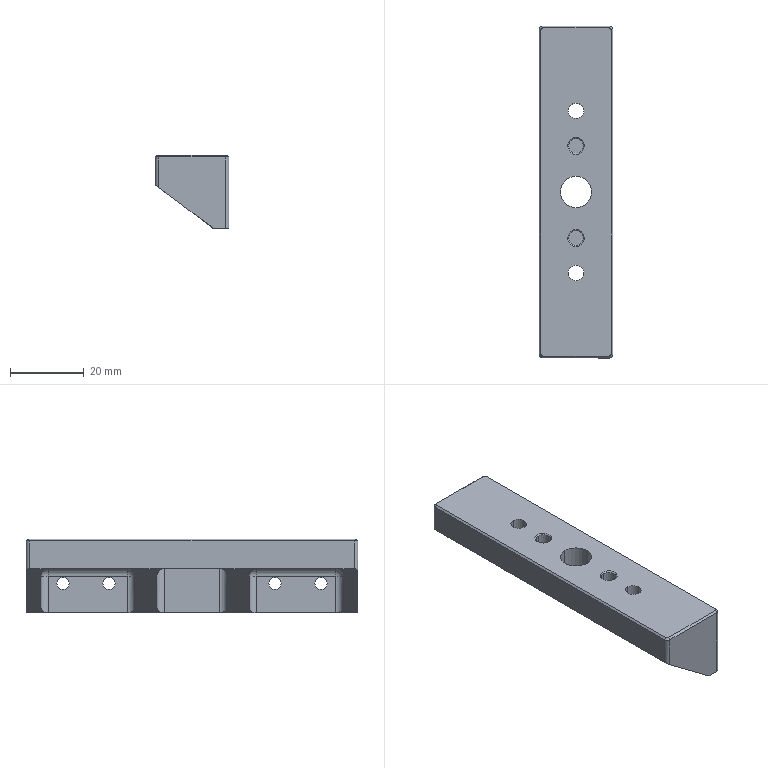NC program | NX | posted with a generic post | part box 20 x 90 x 20 mm
Whole program:
N10 G17 G21 G94 G90
(FLOOR_WALL , TOOL : D80)
N12 T19 M6
N14 G54
N16 G17 G0 G90 X93. Y0. B0. C0. S6500 M3
N18 G43 Z30. H19
N20 Z3.
N22 G94 G1 Z0. F1500.
N24 X90.
N26 X-90.
N28 X-93.
N30 Z3.
N32 G0 Z30.
N34 M5
(DRILLING_COPY_1 , TOOL : D6A45)
N36 T01 M6
N38 G54
N40 G17 G0 G90 X-22. Y0. B0. C0. S5000 M3
N42 G43 Z30. H1
N44 G94 G81 G98 Z-2.3 F350. R3.
N46 X-12.5
N48 X0.
N50 X12.5
N52 X22.
N54 G80
N56 G0 X22. Y0. Z30.
N58 M5
(DRILLING_COPY_COPY , TOOL : 4.2ZT)
N60 T04 M6
N62 G54
N64 G17 G0 G90 X-22. Y0. B0. C0. S2000 M3
N66 G43 Z30. H4
N68 G94 G83 G98 Z-12.262 F180. Q2. R3.
N70 X22.
N72 G80
N74 G0 X22. Y0. Z30.
N76 M5
(ADAPTIVE_MILLING , TOOL : D10)
N78 T15 M6
N80 G54
N82 G17 G0 G90 X0.062 Y-22.709 B0. C0. S9500 M3
N84 G43 Z30. H15
N86 Z-17.
N88 G94 G1 Z-20. F1000.
N90 X0.341 Y-21.928 F3000.
N92 X0.598 Y-21.14
N94 G3 X0.062 Y-20.062 R1.017
N96 X-3.002 Y-19.301 R8.28
N98 X-12.869 Y-19.018 R111.643
N100 G1 X-15.119 Y-19.014
N102 X-18.994 Y-19.011
N104 X-32.619 Y-19.01
N106 X-46.869
N108 X-46.994 Y-19.009
N110 X-47.119 Y-19.007
N112 G2 X-51.4 Y-16.514 R5.714
N114 X-53.465 Y-11.074 R12.318
N116 X-53.953 Y-2.971 R57.395
N118 X-53.956 Y12.528 R542.605
N120 X-51.057 Y16.709 R6.079
N122 X-45.402 Y18.564 R13.739
N124 X-36.541 Y18.967 R76.862
N126 G1 X-35.166 Y18.975
N128 X-33.416 Y18.981
N130 X-30.791 Y18.985
N132 X-25.916 Y18.987
N134 X46.959 Y18.988
N136 X47.084 Y18.987
N138 G2 X51.303 Y16.62 R5.659
N140 X53.46 Y11.087 R12.126
N142 X53.952 Y2.985 R56.695
N144 X53.957 Y-12.514 R598.469
N146 X51.067 Y-16.7 R6.069
N148 X45.414 Y-18.561 R13.651
N150 X36.679 Y-18.965 R74.648
N152 G1 X35.304 Y-18.974
N154 X33.554 Y-18.98
N156 X31.054 Y-18.985
N158 X26.554 Y-18.987
N160 X3.804 Y-18.988
N162 X3.679 Y-18.987
N164 G2 X-1.917 Y-18.439 R78.95
N166 G3 X-14.656 Y-18.033 R144.53
N168 G1 X-16.906 Y-18.027
N170 X-20.156 Y-18.023
N172 X-26.656 Y-18.021
N174 X-43.906 Y-18.02
N176 X-44.031 Y-18.019
N178 X-44.156 Y-18.016
N180 G2 X-50.337 Y-14.316 R7.67
N182 X-52.487 Y-7.845 R15.641
N184 X-52.943 Y1.013 R73.919
N186 X-52.943 Y9.637 R305.783
N188 X-49.084 Y15.462 R7.751
N190 X-42.579 Y17.519 R16.188
N192 X-32.594 Y17.955 R89.291
N194 G1 X-31.094 Y17.963
N196 X-29.219 Y17.969
N198 X-26.469 Y17.974
N200 X-21.594 Y17.977
N202 X9.281
N204 X43.906
N206 G2 X50.268 Y14.382 R7.604
N208 X52.435 Y8.178 R15.104
N210 X52.939 Y-0.676 R69.355
N212 X52.939 Y-9.674 R239.891
N214 X49.05 Y-15.483 R7.794
N216 X42.662 Y-17.507 R16.227
N218 X32.678 Y-17.954 R86.747
N220 G1 X31.178 Y-17.963
N222 X29.303 Y-17.969
N224 X26.553 Y-17.974
N226 X21.678 Y-17.977
N228 X6.178
N230 X5.803 Y-17.975
N232 G2 X-2.176 Y-17.427 R143.365
N234 G3 X-17.043 Y-17.042 R212.317
N236 G1 X-19.668 Y-17.037
N238 X-23.418 Y-17.033
N240 X-31.918 Y-17.031
N242 X-40.918
N244 X-41.293 Y-17.029
N246 X-41.418 Y-17.027
N248 G2 X-49.405 Y-12.311 R8.962
N250 X-51.512 Y-5.168 R18.368
N252 X-51.894 Y7.567 R100.592
N254 X-47.342 Y14.36 R8.873
N256 X-40.583 Y16.456 R17.795
N258 X-30.725 Y16.934 R86.239
N260 G1 X-29.35 Y16.944
N262 X-27.6 Y16.953
N264 X-25.6 Y16.959
N266 X-22.475 Y16.964
N268 X-16.6 Y16.966
N270 X41.275 Y16.967
N272 X41.525 Y16.964
N274 X41.65 Y16.962
N276 X41.775 Y16.959
N278 X41.9 Y16.954
N280 X42.149 Y16.942
N282 G2 X49.399 Y12.277 R8.916
N284 X51.482 Y5.384 R18.11
N286 X51.936 Y-4.475 R91.725
N288 X51.758 Y-8.462 R19.682
N290 X47.095 Y-14.497 R9.036
N292 X40.177 Y-16.504 R18.672
N294 X29.441 Y-16.944 R101.42
N296 G1 X27.816 Y-16.952
N298 X25.816 Y-16.959
N300 X22.816 Y-16.963
N302 X17.441 Y-16.966
N304 X7.941 Y-16.967
N306 X7.441 Y-16.964
N308 G2 X-2.542 Y-16.408 R191.76
N310 G3 X-21.411 Y-16.048 R337.026
N312 G1 X-25.536 Y-16.044
N314 X-34.411 Y-16.042
N316 X-37.911
N318 X-38.661 Y-16.037
N320 X-39.161 Y-16.032
N322 X-39.536 Y-16.024
N324 X-39.66 Y-16.02
N326 G2 X-43.674 Y-15.179 R10.927
N328 G1 X-43.796 Y-15.155
N330 X-43.835 Y-15.15
N332 X-43.97
N334 X-44.03 Y-15.147
N336 X-45.309 Y-15.002
N338 X-45.425 Y-14.976
N340 G2 X-50.002 Y-10.309 R6.283
N342 X-50.873 Y5.252 R122.759
N344 X-50.165 Y8.538 R11.154
N346 X-49.509 Y11.719 R7.514
N348 X-45.309 Y15.002 R6.352
N350 X-26.872 Y15.937 R153.37
N352 G1 X-24.997 Y15.944
N354 X-22.622 Y15.95
N356 X-18.997 Y15.954
N358 X-11.372 Y15.956
N360 X38.878
N362 X39.128 Y15.955
N364 G2 X43.654 Y15.157 R12.961
N366 X47.784 Y13.84 R6.76
N368 X50.147 Y9.03 R6.392
N370 X50.872 Y-5.252 R121.09
N372 X50.164 Y-8.538 R11.16
N374 X49.509 Y-11.719 R7.496
N376 X45.309 Y-15.002 R6.352
N378 X27.873 Y-15.932 R145.512
N380 G1 X26.498 Y-15.94
N382 X24.373 Y-15.947
N384 X21.373 Y-15.952
N386 X16.498 Y-15.955
N388 X9.373 Y-15.956
N390 X8.623 Y-15.951
N392 G2 X-1.24 Y-15.489 R203.518
N394 G3 X-10.193 Y-15.15 R309.747
N396 G1 X-43.943
N398 X-45.309 Y-15.002
N400 X-46.021 Y-14.775
N402 X-46.719 Y-14.509
N404 X-47.784 Y-13.84
N406 X-48.326 Y-13.326
N408 X-48.84 Y-12.784
N410 X-49.509 Y-11.719
N412 X-49.775 Y-11.021
N414 X-50.002 Y-10.309
N416 X-50.15 Y-8.97
N418 Y8.655
N420 X-50.147 Y9.03
N422 X-50.002 Y10.309
N424 X-49.775 Y11.021
N426 X-49.509 Y11.719
N428 X-48.84 Y12.784
N430 X-48.326 Y13.326
N432 X-47.784 Y13.84
N434 X-46.719 Y14.509
N436 X-46.021 Y14.775
N438 X-45.309 Y15.002
N440 X-43.97 Y15.15
N442 X43.78
N444 X44.03 Y15.147
N446 X45.309 Y15.002
N448 X46.021 Y14.775
N450 X46.719 Y14.509
N452 X47.784 Y13.84
N454 X48.326 Y13.326
N456 X48.84 Y12.784
N458 X49.509 Y11.719
N460 X49.775 Y11.021
N462 X50.002 Y10.309
N464 X50.15 Y8.97
N466 Y-8.655
N468 X50.147 Y-9.03
N470 X50.002 Y-10.309
N472 X49.775 Y-11.021
N474 X49.509 Y-11.719
N476 X48.84 Y-12.784
N478 X48.326 Y-13.326
N480 X47.784 Y-13.84
N482 X46.719 Y-14.509
N484 X46.021 Y-14.775
N486 X45.309 Y-15.002
N488 X43.97 Y-15.15
N490 X-10.28
N492 G3 X-11.278 Y-16.003 R1.016
N494 G1 X-11.526 Y-17.587
N496 Z-17.
N498 G0 Z30.
N500 M5
(ZLEVEL_PROFILE_COPY_1_COPY_COPY_1 , TOOL : D10JING)
N502 T14 M6
N504 G54
N506 G17 G0 G90 X45.635 Y-16.831 B0. C0. S9500 M3
N508 G43 Z30. H14
N510 Z-19.
N512 G94 G1 Z-20. F1000.
N514 X44.866 Y-15.5
N516 G3 X44. Y-15. R1.
N518 G1 X-44. F1200.
N520 G2 X-50. Y-9. R6.
N522 G1 Y9.
N524 G2 X-44. Y15. R6.
N526 G1 X44.
N528 G2 X50. Y9. R6.
N530 G1 Y-9.
N532 G2 X44. Y-15. R6.
N534 G3 X43.134 Y-15.5 R1.
N536 G1 X42.268 Y-17.
N538 Z-19.
N540 G0 Z30.
N542 M5
(HOLE_MILLING , TOOL : D6)
N544 T12 M6
N546 G54
N548 G17 G0 G90 X0. Y0. B0. C0. S9500 M3
N550 G43 Z30. H12
N552 Z0.5
N554 G94 G3 X0.625 Y0.625 R0.625 F1500.
N556 X0. Y1.25 R0.625
N558 X0. Y1.25 Z0. I0. J-1.25
N560 X0. Y1.25 Z-0.5 I0. J-1.25
N562 X0. Y1.25 Z-1. I0. J-1.25
N564 X0. Y1.25 Z-1.5 I0. J-1.25
N566 X0. Y1.25 Z-2. I0. J-1.25
N568 X0. Y1.25 Z-2.5 I0. J-1.25
N570 X0. Y1.25 Z-3. I0. J-1.25
N572 X0. Y1.25 Z-3.5 I0. J-1.25
N574 X0. Y1.25 Z-4. I0. J-1.25
N576 X0. Y1.25 Z-4.5 I0. J-1.25
N578 X0. Y1.25 Z-5. I0. J-1.25
N580 X0. Y1.25 Z-5.5 I0. J-1.25
N582 X0. Y1.25 Z-6. I0. J-1.25
N584 X0. Y1.25 Z-6.5 I0. J-1.25
N586 X0. Y1.25 Z-7. I0. J-1.25
N588 X0. Y1.25 Z-7.5 I0. J-1.25
N590 X0. Y1.25 Z-8. I0. J-1.25
N592 X-1.25 Y0. R1.25
N594 X0. Y1.25 R-1.25
N596 X-0.625 Y0.625 R0.625
N598 X0. Y0. R0.625
N600 G0 Z30.
N602 M5
(HOLE_MILLING_COPY , TOOL : D3)
N604 T17 M6
N606 G54
N608 G17 G0 G90 X-12.5 Y0. B0. C0. S9500 M3
N610 G43 Z30. H17
N612 Z0.5
N614 G94 G3 X-12.3 Y0.2 R0.2 F1200.
N616 X-12.5 Y0.4 R0.2
N618 X-12.5 Y0.4 Z0.25 I0. J-0.4
N620 X-12.5 Y0.4 Z0. I0. J-0.4
N622 X-12.5 Y0.4 Z-0.25 I0. J-0.4
N624 X-12.5 Y0.4 Z-0.5 I0. J-0.4
N626 X-12.5 Y0.4 Z-0.75 I0. J-0.4
N628 X-12.5 Y0.4 Z-1. I0. J-0.4
N630 X-12.5 Y0.4 Z-1.25 I0. J-0.4
N632 X-12.5 Y0.4 Z-1.5 I0. J-0.4
N634 X-12.5 Y0.4 Z-1.75 I0. J-0.4
N636 X-12.5 Y0.4 Z-2. I0. J-0.4
N638 X-12.5 Y0.4 Z-2.25 I0. J-0.4
N640 X-12.5 Y0.4 Z-2.5 I0. J-0.4
N642 X-12.5 Y0.4 Z-2.75 I0. J-0.4
N644 X-12.5 Y0.4 Z-3. I0. J-0.4
N646 X-12.5 Y0.4 Z-3.25 I0. J-0.4
N648 X-12.5 Y0.4 Z-3.5 I0. J-0.4
N650 X-12.5 Y0.4 Z-3.75 I0. J-0.4
N652 X-12.5 Y0.4 Z-4. I0. J-0.4
N654 X-12.5 Y0.4 Z-4.25 I0. J-0.4
N656 X-12.5 Y0.4 Z-4.5 I0. J-0.4
N658 X-12.5 Y0.4 Z-4.75 I0. J-0.4
N660 X-12.5 Y0.4 Z-5. I0. J-0.4
N662 X-12.5 Y0.4 Z-5.25 I0. J-0.4
N664 X-12.5 Y0.4 Z-5.5 I0. J-0.4
N666 X-12.5 Y0.4 Z-5.75 I0. J-0.4
N668 X-12.5 Y0.4 Z-6. I0. J-0.4
N670 X-12.9 Y0. R0.4
N672 X-12.5 Y0.4 R-0.4
N674 X-12.7 Y0.2 R0.2
N676 X-12.5 Y0. R0.2
N678 G0 Z30.
N680 X12.5
N682 Z0.5
N684 G3 X12.7 Y0.2 R0.2
N686 X12.5 Y0.4 R0.2
N688 X12.5 Y0.4 Z0.25 I0. J-0.4
N690 X12.5 Y0.4 Z0. I0. J-0.4
N692 X12.5 Y0.4 Z-0.25 I0. J-0.4
N694 X12.5 Y0.4 Z-0.5 I0. J-0.4
N696 X12.5 Y0.4 Z-0.75 I0. J-0.4
N698 X12.5 Y0.4 Z-1. I0. J-0.4
N700 X12.5 Y0.4 Z-1.25 I0. J-0.4
N702 X12.5 Y0.4 Z-1.5 I0. J-0.4
N704 X12.5 Y0.4 Z-1.75 I0. J-0.4
N706 X12.5 Y0.4 Z-2. I0. J-0.4
N708 X12.5 Y0.4 Z-2.25 I0. J-0.4
N710 X12.5 Y0.4 Z-2.5 I0. J-0.4
N712 X12.5 Y0.4 Z-2.75 I0. J-0.4
N714 X12.5 Y0.4 Z-3. I0. J-0.4
N716 X12.5 Y0.4 Z-3.25 I0. J-0.4
N718 X12.5 Y0.4 Z-3.5 I0. J-0.4
N720 X12.5 Y0.4 Z-3.75 I0. J-0.4
N722 X12.5 Y0.4 Z-4. I0. J-0.4
N724 X12.5 Y0.4 Z-4.25 I0. J-0.4
N726 X12.5 Y0.4 Z-4.5 I0. J-0.4
N728 X12.5 Y0.4 Z-4.75 I0. J-0.4
N730 X12.5 Y0.4 Z-5. I0. J-0.4
N732 X12.5 Y0.4 Z-5.25 I0. J-0.4
N734 X12.5 Y0.4 Z-5.5 I0. J-0.4
N736 X12.5 Y0.4 Z-5.75 I0. J-0.4
N738 X12.5 Y0.4 Z-6. I0. J-0.4
N740 X12.1 Y0. R0.4
N742 X12.5 Y0.4 R-0.4
N744 X12.3 Y0.2 R0.2
N746 X12.5 Y0. R0.2
N748 G0 Z30.
N750 M5
(PLANAR_MILL_COPY_COPY_COPY_COPY_COPY_COPY_1 , TOOL : D6A45)
N752 T01 M6
N754 G54
N756 G17 G0 G90 X0.866 Y-10.9 B0. C0. S9500 M3
N758 G43 Z30. H1
N760 Z0.5
N762 G94 G1 Z-1. F1250.
N764 G3 X0. Y-10.4 R1.
N766 G1 X-44.
N768 G2 X-45.4 Y-9. R1.4
N770 G1 Y9.
N772 G2 X-44. Y10.4 R1.4
N774 G1 X44.
N776 G2 X45.4 Y9. R1.4
N778 G1 Y-9.
N780 G2 X44. Y-10.4 R1.4
N782 G1 X0.
N784 G3 X-0.866 Y-10.9 R1.
N786 G1 Z0.5
N788 G0 Z30.
N790 M5
(HOLE_MILLING_COPY_COPY , TOOL : D3)
N792 T17 M6
N794 G54
N796 G17 G0 G90 X-12.5 Y0. B0. C0. S9500 M3
N798 G43 Z30. H17
N800 Z0.5
N802 G41 G94 G1 X-12.404 Y0.027 F1200. D17
N804 G3 X-12.5 Y0.45 R0.222
N806 X-12.5 Y0.45 Z-2.5 I0. J-0.45
N808 X-12.5 Y0.45 Z-5.5 I0. J-0.45
N810 X-12.89 Y0.225 Z-6. R0.45
N812 X-12.725 Y-0.39 R0.45
N814 X-12.89 Y0.225 R-0.45
N816 X-12.572 Y-0.07 R0.222
N818 G40
N820 G1 X-12.5 Y0.
N822 G0 Z30.
N824 X12.5
N826 Z0.5
N828 G41 G1 X12.596 Y0.027
N830 G3 X12.5 Y0.45 R0.222
N832 X12.5 Y0.45 Z-2.5 I0. J-0.45
N834 X12.5 Y0.45 Z-5.5 I0. J-0.45
N836 X12.11 Y0.225 Z-6. R0.45
N838 X12.275 Y-0.39 R0.45
N840 X12.11 Y0.225 R-0.45
N842 X12.428 Y-0.07 R0.222
N844 G40
N846 G1 X12.5 Y0.
N848 G0 Z30.
N850 M5
N852 M2